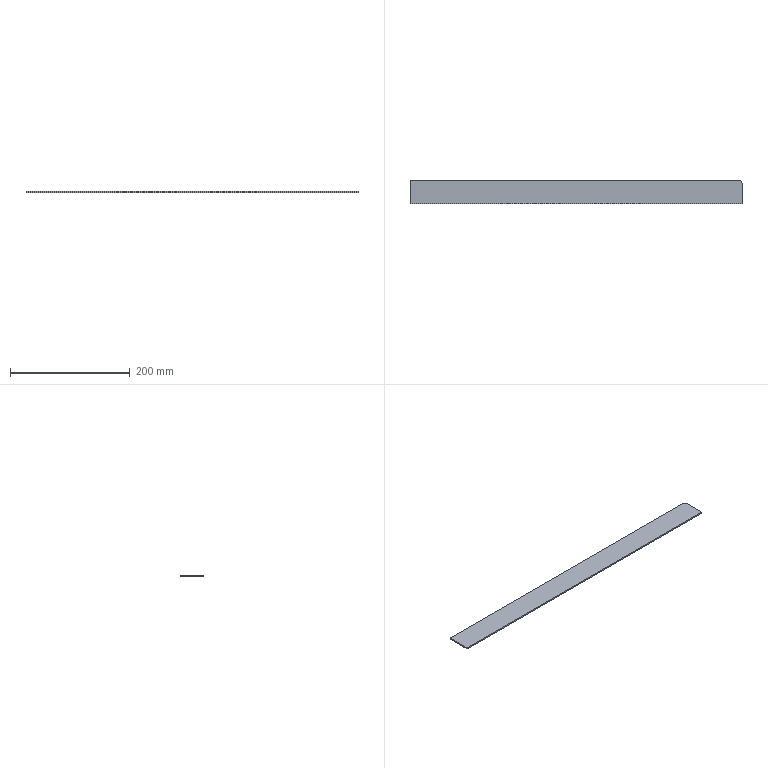Part | SolidWorks | features FlatPattern 1, SMBaseFlange 1, SheetMetal 1 | 1 solid | 7 faces | box 554 x 40 x 2.3 mm | volume 50956 mm3 | plane 6 | cylinder 1 | commonest cylinder face diameters 10 x1
STEP:
#1=CARTESIAN_POINT('',(0.,0.,0.));
#2=VERTEX_POINT('',#1);
#3=CARTESIAN_POINT('',(0.,-40.,0.));
#4=VERTEX_POINT('',#3);
#5=CARTESIAN_POINT('',(0.,0.,0.));
#6=DIRECTION('',(0.,-1.,0.));
#7=VECTOR('',#6,1000.);
#8=LINE('',#5,#7);
#9=EDGE_CURVE('',#2,#4,#8,.T.);
#10=ORIENTED_EDGE('',*,*,#9,.F.);
#11=CARTESIAN_POINT('',(0.,0.,-2.3));
#12=VERTEX_POINT('',#11);
#13=CARTESIAN_POINT('',(0.,0.,-2.3));
#14=DIRECTION('',(0.,0.,1.));
#15=VECTOR('',#14,1000.);
#16=LINE('',#13,#15);
#17=EDGE_CURVE('',#12,#2,#16,.T.);
#18=ORIENTED_EDGE('',*,*,#17,.F.);
#19=CARTESIAN_POINT('',(0.,-40.,-2.3));
#20=VERTEX_POINT('',#19);
#21=CARTESIAN_POINT('',(0.,0.,-2.3));
#22=DIRECTION('',(0.,-1.,0.));
#23=VECTOR('',#22,1000.);
#24=LINE('',#21,#23);
#25=EDGE_CURVE('',#12,#20,#24,.T.);
#26=ORIENTED_EDGE('',*,*,#25,.T.);
#27=CARTESIAN_POINT('',(0.,-40.,-2.3));
#28=DIRECTION('',(0.,0.,1.));
#29=VECTOR('',#28,1000.);
#30=LINE('',#27,#29);
#31=EDGE_CURVE('',#20,#4,#30,.T.);
#32=ORIENTED_EDGE('',*,*,#31,.T.);
#33=EDGE_LOOP('',(#10,#18,#26,#32));
#34=FACE_OUTER_BOUND('',#33,.T.);
#35=CARTESIAN_POINT('',(0.,0.,-2.3));
#36=DIRECTION('',(-1.,0.,0.));
#37=DIRECTION('',(0.,0.,1.));
#38=AXIS2_PLACEMENT_3D('',#35,#36,#37);
#39=PLANE('',#38);
#40=ADVANCED_FACE('',(#34),#39,.T.);
#41=CARTESIAN_POINT('',(549.,0.,0.));
#42=VERTEX_POINT('',#41);
#43=CARTESIAN_POINT('',(0.,0.,0.));
#44=DIRECTION('',(-1.,0.,0.));
#45=VECTOR('',#44,1000.);
#46=LINE('',#43,#45);
#47=EDGE_CURVE('',#42,#2,#46,.T.);
#48=ORIENTED_EDGE('',*,*,#47,.F.);
#49=CARTESIAN_POINT('',(549.,0.,-2.3));
#50=VERTEX_POINT('',#49);
#51=CARTESIAN_POINT('',(549.,0.,-2.3));
#52=DIRECTION('',(0.,0.,1.));
#53=VECTOR('',#52,1000.);
#54=LINE('',#51,#53);
#55=EDGE_CURVE('',#50,#42,#54,.T.);
#56=ORIENTED_EDGE('',*,*,#55,.F.);
#57=CARTESIAN_POINT('',(0.,0.,-2.3));
#58=DIRECTION('',(-1.,0.,0.));
#59=VECTOR('',#58,1000.);
#60=LINE('',#57,#59);
#61=EDGE_CURVE('',#50,#12,#60,.T.);
#62=ORIENTED_EDGE('',*,*,#61,.T.);
#63=ORIENTED_EDGE('',*,*,#17,.T.);
#64=EDGE_LOOP('',(#48,#56,#62,#63));
#65=FACE_OUTER_BOUND('',#64,.T.);
#66=CARTESIAN_POINT('',(0.,0.,-2.3));
#67=DIRECTION('',(0.,1.,0.));
#68=DIRECTION('',(0.,0.,1.));
#69=AXIS2_PLACEMENT_3D('',#66,#67,#68);
#70=PLANE('',#69);
#71=ADVANCED_FACE('',(#65),#70,.T.);
#72=CARTESIAN_POINT('',(554.,-5.,0.));
#73=VERTEX_POINT('',#72);
#74=CARTESIAN_POINT('',(549.,-5.,0.));
#75=DIRECTION('',(0.,0.,1.));
#76=DIRECTION('',(-1.,0.,0.));
#77=AXIS2_PLACEMENT_3D('',#74,#75,#76);
#78=CIRCLE('',#77,5.);
#79=EDGE_CURVE('',#73,#42,#78,.T.);
#80=ORIENTED_EDGE('',*,*,#79,.F.);
#81=CARTESIAN_POINT('',(554.,-5.,-2.3));
#82=VERTEX_POINT('',#81);
#83=CARTESIAN_POINT('',(554.,-5.,-2.3));
#84=DIRECTION('',(0.,0.,1.));
#85=VECTOR('',#84,1000.);
#86=LINE('',#83,#85);
#87=EDGE_CURVE('',#82,#73,#86,.T.);
#88=ORIENTED_EDGE('',*,*,#87,.F.);
#89=CARTESIAN_POINT('',(549.,-5.,-2.3));
#90=DIRECTION('',(0.,0.,1.));
#91=DIRECTION('',(-1.,0.,0.));
#92=AXIS2_PLACEMENT_3D('',#89,#90,#91);
#93=CIRCLE('',#92,5.);
#94=EDGE_CURVE('',#82,#50,#93,.T.);
#95=ORIENTED_EDGE('',*,*,#94,.T.);
#96=ORIENTED_EDGE('',*,*,#55,.T.);
#97=EDGE_LOOP('',(#80,#88,#95,#96));
#98=FACE_OUTER_BOUND('',#97,.T.);
#99=CARTESIAN_POINT('',(549.,-5.,-2.3));
#100=DIRECTION('',(0.,0.,1.));
#101=DIRECTION('',(1.,0.,0.));
#102=AXIS2_PLACEMENT_3D('',#99,#100,#101);
#103=CYLINDRICAL_SURFACE('',#102,5.);
#104=ADVANCED_FACE('',(#98),#103,.T.);
#105=CARTESIAN_POINT('',(554.,-40.,0.));
#106=VERTEX_POINT('',#105);
#107=CARTESIAN_POINT('',(554.,-5.,0.));
#108=DIRECTION('',(0.,1.,0.));
#109=VECTOR('',#108,1000.);
#110=LINE('',#107,#109);
#111=EDGE_CURVE('',#106,#73,#110,.T.);
#112=ORIENTED_EDGE('',*,*,#111,.F.);
#113=CARTESIAN_POINT('',(554.,-40.,-2.3));
#114=VERTEX_POINT('',#113);
#115=CARTESIAN_POINT('',(554.,-40.,-2.3));
#116=DIRECTION('',(0.,0.,1.));
#117=VECTOR('',#116,1000.);
#118=LINE('',#115,#117);
#119=EDGE_CURVE('',#114,#106,#118,.T.);
#120=ORIENTED_EDGE('',*,*,#119,.F.);
#121=CARTESIAN_POINT('',(554.,-5.,-2.3));
#122=DIRECTION('',(0.,1.,0.));
#123=VECTOR('',#122,1000.);
#124=LINE('',#121,#123);
#125=EDGE_CURVE('',#114,#82,#124,.T.);
#126=ORIENTED_EDGE('',*,*,#125,.T.);
#127=ORIENTED_EDGE('',*,*,#87,.T.);
#128=EDGE_LOOP('',(#112,#120,#126,#127));
#129=FACE_OUTER_BOUND('',#128,.T.);
#130=CARTESIAN_POINT('',(554.,-5.,-2.3));
#131=DIRECTION('',(1.,0.,0.));
#132=DIRECTION('',(0.,0.,-1.));
#133=AXIS2_PLACEMENT_3D('',#130,#131,#132);
#134=PLANE('',#133);
#135=ADVANCED_FACE('',(#129),#134,.T.);
#136=CARTESIAN_POINT('',(0.,-40.,0.));
#137=DIRECTION('',(1.,0.,0.));
#138=VECTOR('',#137,1000.);
#139=LINE('',#136,#138);
#140=EDGE_CURVE('',#4,#106,#139,.T.);
#141=ORIENTED_EDGE('',*,*,#140,.F.);
#142=ORIENTED_EDGE('',*,*,#31,.F.);
#143=CARTESIAN_POINT('',(0.,-40.,-2.3));
#144=DIRECTION('',(1.,0.,0.));
#145=VECTOR('',#144,1000.);
#146=LINE('',#143,#145);
#147=EDGE_CURVE('',#20,#114,#146,.T.);
#148=ORIENTED_EDGE('',*,*,#147,.T.);
#149=ORIENTED_EDGE('',*,*,#119,.T.);
#150=EDGE_LOOP('',(#141,#142,#148,#149));
#151=FACE_OUTER_BOUND('',#150,.T.);
#152=CARTESIAN_POINT('',(0.,-40.,-2.3));
#153=DIRECTION('',(0.,-1.,0.));
#154=DIRECTION('',(0.,0.,-1.));
#155=AXIS2_PLACEMENT_3D('',#152,#153,#154);
#156=PLANE('',#155);
#157=ADVANCED_FACE('',(#151),#156,.T.);
#158=ORIENTED_EDGE('',*,*,#25,.F.);
#159=ORIENTED_EDGE('',*,*,#61,.F.);
#160=ORIENTED_EDGE('',*,*,#94,.F.);
#161=ORIENTED_EDGE('',*,*,#125,.F.);
#162=ORIENTED_EDGE('',*,*,#147,.F.);
#163=EDGE_LOOP('',(#158,#159,#160,#161,#162));
#164=FACE_OUTER_BOUND('',#163,.T.);
#165=CARTESIAN_POINT('',(549.,-5.,-2.3));
#166=DIRECTION('',(0.,0.,-1.));
#167=DIRECTION('',(-1.,0.,0.));
#168=AXIS2_PLACEMENT_3D('',#165,#166,#167);
#169=PLANE('',#168);
#170=ADVANCED_FACE('',(#164),#169,.T.);
#171=ORIENTED_EDGE('',*,*,#9,.T.);
#172=ORIENTED_EDGE('',*,*,#140,.T.);
#173=ORIENTED_EDGE('',*,*,#111,.T.);
#174=ORIENTED_EDGE('',*,*,#79,.T.);
#175=ORIENTED_EDGE('',*,*,#47,.T.);
#176=EDGE_LOOP('',(#171,#172,#173,#174,#175));
#177=FACE_OUTER_BOUND('',#176,.T.);
#178=CARTESIAN_POINT('',(549.,-5.,0.));
#179=DIRECTION('',(0.,0.,-1.));
#180=DIRECTION('',(-1.,0.,0.));
#181=AXIS2_PLACEMENT_3D('',#178,#179,#180);
#182=PLANE('',#181);
#183=ADVANCED_FACE('',(#177),#182,.F.);
#184=CLOSED_SHELL('',(#40,#71,#104,#135,#157,#170,#183));
#185=MANIFOLD_SOLID_BREP('',#184);
#186=CARTESIAN_POINT('',(0.,0.,0.));
#187=DIRECTION('',(0.,0.,1.));
#188=DIRECTION('',(1.,0.,0.));
#189=AXIS2_PLACEMENT_3D('',#186,#187,#188);
#190=(LENGTH_UNIT()NAMED_UNIT(*)SI_UNIT(.MILLI.,.METRE.));
#191=UNCERTAINTY_MEASURE_WITH_UNIT(LENGTH_MEASURE(0.00001),#190,'','');
#192=(NAMED_UNIT(*)PLANE_ANGLE_UNIT()SI_UNIT($,.RADIAN.));
#193=(NAMED_UNIT(*)SI_UNIT($,.STERADIAN.)SOLID_ANGLE_UNIT());
#194=(GEOMETRIC_REPRESENTATION_CONTEXT(3)GLOBAL_UNCERTAINTY_ASSIGNED_CONTEXT((#191))GLOBAL_UNIT_ASSIGNED_CONTEXT((#190,#192,#193))REPRESENTATION_CONTEXT('',''));
#195=ADVANCED_BREP_SHAPE_REPRESENTATION('',(#185,#189),#194);